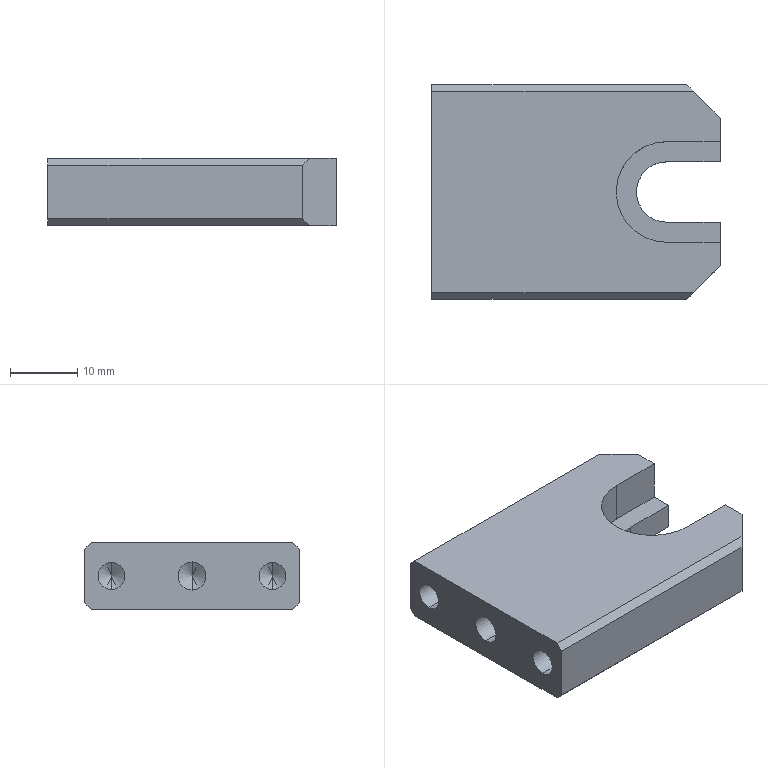Part | STEP file | QA-AD14 | 1 solid | 32 faces | box 43 x 32 x 10 mm | volume 11347 mm3 | plane 18 | cylinder 8 | cone 6 | commonest cylinder face diameters 4 x4 4.2 x2 9 x1 15 x1